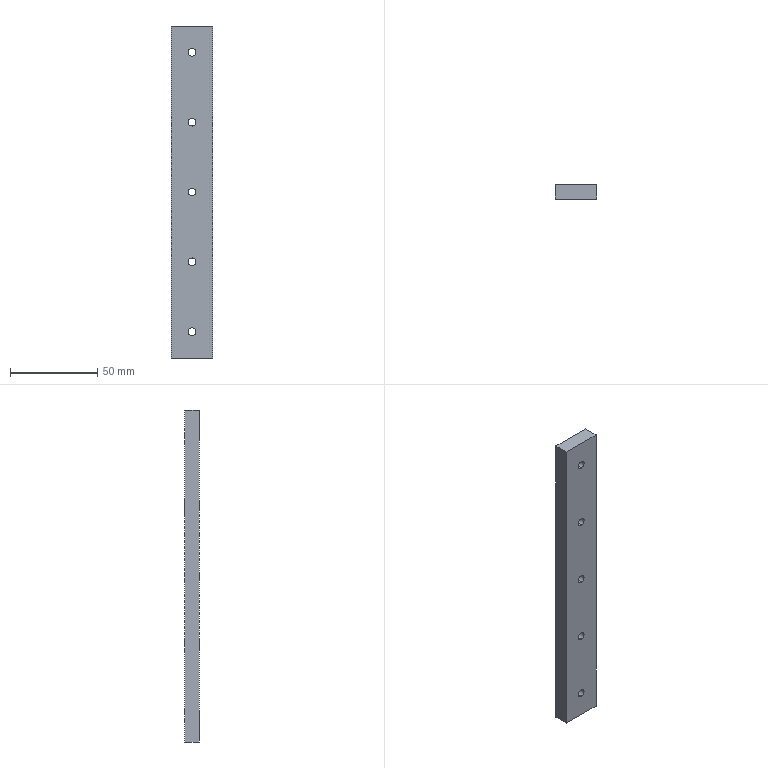Part | STEP file | 11-MGW12CR190Z0C11 | 1 solid | 31 faces | box 24 x 8.5 x 190 mm | volume 37397 mm3 | cylinder 20 | plane 11 | commonest cylinder face diameters 4.5 x10 8 x10
STEP:
#1=CARTESIAN_POINT('',(-44.741,27.003,12.75));
#2=VERTEX_POINT('',#1);
#3=CARTESIAN_POINT('',(-44.741,27.003,17.25));
#4=VERTEX_POINT('',#3);
#5=CARTESIAN_POINT('',(-44.741,27.003,15.));
#6=DIRECTION('',(0.,1.,0.));
#7=DIRECTION('',(0.,0.,1.));
#8=AXIS2_PLACEMENT_3D('',#5,#6,#7);
#9=CIRCLE('',#8,2.25);
#10=EDGE_CURVE('',#2,#4,#9,.T.);
#11=ORIENTED_EDGE('',*,*,#10,.F.);
#12=CARTESIAN_POINT('',(-44.741,31.503,12.75));
#13=VERTEX_POINT('',#12);
#14=CARTESIAN_POINT('',(-44.741,35.503,12.75));
#15=DIRECTION('',(0.,1.,0.));
#16=VECTOR('',#15,1000.);
#17=LINE('',#14,#16);
#18=EDGE_CURVE('',#2,#13,#17,.T.);
#19=ORIENTED_EDGE('',*,*,#18,.T.);
#20=CARTESIAN_POINT('',(-44.741,31.503,17.25));
#21=VERTEX_POINT('',#20);
#22=CARTESIAN_POINT('',(-44.741,31.503,15.));
#23=DIRECTION('',(0.,1.,0.));
#24=DIRECTION('',(0.,0.,1.));
#25=AXIS2_PLACEMENT_3D('',#22,#23,#24);
#26=CIRCLE('',#25,2.25);
#27=EDGE_CURVE('',#13,#21,#26,.T.);
#28=ORIENTED_EDGE('',*,*,#27,.T.);
#29=CARTESIAN_POINT('',(-44.741,35.503,17.25));
#30=DIRECTION('',(0.,1.,0.));
#31=VECTOR('',#30,1000.);
#32=LINE('',#29,#31);
#33=EDGE_CURVE('',#4,#21,#32,.T.);
#34=ORIENTED_EDGE('',*,*,#33,.F.);
#35=EDGE_LOOP('',(#11,#19,#28,#34));
#36=FACE_OUTER_BOUND('',#35,.T.);
#37=CARTESIAN_POINT('',(-44.741,35.503,15.));
#38=DIRECTION('',(0.,1.,0.));
#39=DIRECTION('',(0.,0.,1.));
#40=AXIS2_PLACEMENT_3D('',#37,#38,#39);
#41=CYLINDRICAL_SURFACE('',#40,2.25);
#42=ADVANCED_FACE('',(#36),#41,.F.);
#43=CARTESIAN_POINT('',(-44.741,31.503,11.));
#44=VERTEX_POINT('',#43);
#45=CARTESIAN_POINT('',(-44.741,31.503,19.));
#46=VERTEX_POINT('',#45);
#47=CARTESIAN_POINT('',(-44.741,31.503,15.));
#48=DIRECTION('',(0.,1.,0.));
#49=DIRECTION('',(0.,0.,1.));
#50=AXIS2_PLACEMENT_3D('',#47,#48,#49);
#51=CIRCLE('',#50,4.);
#52=EDGE_CURVE('',#44,#46,#51,.T.);
#53=ORIENTED_EDGE('',*,*,#52,.F.);
#54=CARTESIAN_POINT('',(-44.741,35.503,11.));
#55=VERTEX_POINT('',#54);
#56=CARTESIAN_POINT('',(-44.741,35.503,11.));
#57=DIRECTION('',(0.,1.,0.));
#58=VECTOR('',#57,1000.);
#59=LINE('',#56,#58);
#60=EDGE_CURVE('',#44,#55,#59,.T.);
#61=ORIENTED_EDGE('',*,*,#60,.T.);
#62=CARTESIAN_POINT('',(-44.741,35.503,19.));
#63=VERTEX_POINT('',#62);
#64=CARTESIAN_POINT('',(-44.741,35.503,15.));
#65=DIRECTION('',(0.,1.,0.));
#66=DIRECTION('',(0.,0.,1.));
#67=AXIS2_PLACEMENT_3D('',#64,#65,#66);
#68=CIRCLE('',#67,4.);
#69=EDGE_CURVE('',#55,#63,#68,.T.);
#70=ORIENTED_EDGE('',*,*,#69,.T.);
#71=CARTESIAN_POINT('',(-44.741,35.503,19.));
#72=DIRECTION('',(0.,1.,0.));
#73=VECTOR('',#72,1000.);
#74=LINE('',#71,#73);
#75=EDGE_CURVE('',#46,#63,#74,.T.);
#76=ORIENTED_EDGE('',*,*,#75,.F.);
#77=EDGE_LOOP('',(#53,#61,#70,#76));
#78=FACE_OUTER_BOUND('',#77,.T.);
#79=CARTESIAN_POINT('',(-44.741,35.503,15.));
#80=DIRECTION('',(0.,1.,0.));
#81=DIRECTION('',(0.,0.,1.));
#82=AXIS2_PLACEMENT_3D('',#79,#80,#81);
#83=CYLINDRICAL_SURFACE('',#82,4.);
#84=ADVANCED_FACE('',(#78),#83,.F.);
#85=CARTESIAN_POINT('',(-44.741,27.003,52.75));
#86=VERTEX_POINT('',#85);
#87=CARTESIAN_POINT('',(-44.741,27.003,57.25));
#88=VERTEX_POINT('',#87);
#89=CARTESIAN_POINT('',(-44.741,27.003,55.));
#90=DIRECTION('',(0.,1.,0.));
#91=DIRECTION('',(0.,0.,1.));
#92=AXIS2_PLACEMENT_3D('',#89,#90,#91);
#93=CIRCLE('',#92,2.25);
#94=EDGE_CURVE('',#86,#88,#93,.T.);
#95=ORIENTED_EDGE('',*,*,#94,.F.);
#96=CARTESIAN_POINT('',(-44.741,31.503,52.75));
#97=VERTEX_POINT('',#96);
#98=CARTESIAN_POINT('',(-44.741,35.503,52.75));
#99=DIRECTION('',(0.,1.,0.));
#100=VECTOR('',#99,1000.);
#101=LINE('',#98,#100);
#102=EDGE_CURVE('',#86,#97,#101,.T.);
#103=ORIENTED_EDGE('',*,*,#102,.T.);
#104=CARTESIAN_POINT('',(-44.741,31.503,57.25));
#105=VERTEX_POINT('',#104);
#106=CARTESIAN_POINT('',(-44.741,31.503,55.));
#107=DIRECTION('',(0.,1.,0.));
#108=DIRECTION('',(0.,0.,1.));
#109=AXIS2_PLACEMENT_3D('',#106,#107,#108);
#110=CIRCLE('',#109,2.25);
#111=EDGE_CURVE('',#97,#105,#110,.T.);
#112=ORIENTED_EDGE('',*,*,#111,.T.);
#113=CARTESIAN_POINT('',(-44.741,35.503,57.25));
#114=DIRECTION('',(0.,1.,0.));
#115=VECTOR('',#114,1000.);
#116=LINE('',#113,#115);
#117=EDGE_CURVE('',#88,#105,#116,.T.);
#118=ORIENTED_EDGE('',*,*,#117,.F.);
#119=EDGE_LOOP('',(#95,#103,#112,#118));
#120=FACE_OUTER_BOUND('',#119,.T.);
#121=CARTESIAN_POINT('',(-44.741,35.503,55.));
#122=DIRECTION('',(0.,1.,0.));
#123=DIRECTION('',(0.,0.,1.));
#124=AXIS2_PLACEMENT_3D('',#121,#122,#123);
#125=CYLINDRICAL_SURFACE('',#124,2.25);
#126=ADVANCED_FACE('',(#120),#125,.F.);
#127=CARTESIAN_POINT('',(-44.741,31.503,51.));
#128=VERTEX_POINT('',#127);
#129=CARTESIAN_POINT('',(-44.741,31.503,59.));
#130=VERTEX_POINT('',#129);
#131=CARTESIAN_POINT('',(-44.741,31.503,55.));
#132=DIRECTION('',(0.,1.,0.));
#133=DIRECTION('',(0.,0.,1.));
#134=AXIS2_PLACEMENT_3D('',#131,#132,#133);
#135=CIRCLE('',#134,4.);
#136=EDGE_CURVE('',#128,#130,#135,.T.);
#137=ORIENTED_EDGE('',*,*,#136,.F.);
#138=CARTESIAN_POINT('',(-44.741,35.503,51.));
#139=VERTEX_POINT('',#138);
#140=CARTESIAN_POINT('',(-44.741,35.503,51.));
#141=DIRECTION('',(0.,1.,0.));
#142=VECTOR('',#141,1000.);
#143=LINE('',#140,#142);
#144=EDGE_CURVE('',#128,#139,#143,.T.);
#145=ORIENTED_EDGE('',*,*,#144,.T.);
#146=CARTESIAN_POINT('',(-44.741,35.503,59.));
#147=VERTEX_POINT('',#146);
#148=CARTESIAN_POINT('',(-44.741,35.503,55.));
#149=DIRECTION('',(0.,1.,0.));
#150=DIRECTION('',(0.,0.,1.));
#151=AXIS2_PLACEMENT_3D('',#148,#149,#150);
#152=CIRCLE('',#151,4.);
#153=EDGE_CURVE('',#139,#147,#152,.T.);
#154=ORIENTED_EDGE('',*,*,#153,.T.);
#155=CARTESIAN_POINT('',(-44.741,35.503,59.));
#156=DIRECTION('',(0.,1.,0.));
#157=VECTOR('',#156,1000.);
#158=LINE('',#155,#157);
#159=EDGE_CURVE('',#130,#147,#158,.T.);
#160=ORIENTED_EDGE('',*,*,#159,.F.);
#161=EDGE_LOOP('',(#137,#145,#154,#160));
#162=FACE_OUTER_BOUND('',#161,.T.);
#163=CARTESIAN_POINT('',(-44.741,35.503,55.));
#164=DIRECTION('',(0.,1.,0.));
#165=DIRECTION('',(0.,0.,1.));
#166=AXIS2_PLACEMENT_3D('',#163,#164,#165);
#167=CYLINDRICAL_SURFACE('',#166,4.);
#168=ADVANCED_FACE('',(#162),#167,.F.);
#169=CARTESIAN_POINT('',(-44.741,27.003,92.75));
#170=VERTEX_POINT('',#169);
#171=CARTESIAN_POINT('',(-44.741,27.003,97.25));
#172=VERTEX_POINT('',#171);
#173=CARTESIAN_POINT('',(-44.741,27.003,95.));
#174=DIRECTION('',(0.,1.,0.));
#175=DIRECTION('',(0.,0.,1.));
#176=AXIS2_PLACEMENT_3D('',#173,#174,#175);
#177=CIRCLE('',#176,2.25);
#178=EDGE_CURVE('',#170,#172,#177,.T.);
#179=ORIENTED_EDGE('',*,*,#178,.F.);
#180=CARTESIAN_POINT('',(-44.741,31.503,92.75));
#181=VERTEX_POINT('',#180);
#182=CARTESIAN_POINT('',(-44.741,35.503,92.75));
#183=DIRECTION('',(0.,1.,0.));
#184=VECTOR('',#183,1000.);
#185=LINE('',#182,#184);
#186=EDGE_CURVE('',#170,#181,#185,.T.);
#187=ORIENTED_EDGE('',*,*,#186,.T.);
#188=CARTESIAN_POINT('',(-44.741,31.503,97.25));
#189=VERTEX_POINT('',#188);
#190=CARTESIAN_POINT('',(-44.741,31.503,95.));
#191=DIRECTION('',(0.,1.,0.));
#192=DIRECTION('',(0.,0.,1.));
#193=AXIS2_PLACEMENT_3D('',#190,#191,#192);
#194=CIRCLE('',#193,2.25);
#195=EDGE_CURVE('',#181,#189,#194,.T.);
#196=ORIENTED_EDGE('',*,*,#195,.T.);
#197=CARTESIAN_POINT('',(-44.741,35.503,97.25));
#198=DIRECTION('',(0.,1.,0.));
#199=VECTOR('',#198,1000.);
#200=LINE('',#197,#199);
#201=EDGE_CURVE('',#172,#189,#200,.T.);
#202=ORIENTED_EDGE('',*,*,#201,.F.);
#203=EDGE_LOOP('',(#179,#187,#196,#202));
#204=FACE_OUTER_BOUND('',#203,.T.);
#205=CARTESIAN_POINT('',(-44.741,35.503,95.));
#206=DIRECTION('',(0.,1.,0.));
#207=DIRECTION('',(0.,0.,1.));
#208=AXIS2_PLACEMENT_3D('',#205,#206,#207);
#209=CYLINDRICAL_SURFACE('',#208,2.25);
#210=ADVANCED_FACE('',(#204),#209,.F.);
#211=CARTESIAN_POINT('',(-44.741,31.503,91.));
#212=VERTEX_POINT('',#211);
#213=CARTESIAN_POINT('',(-44.741,31.503,99.));
#214=VERTEX_POINT('',#213);
#215=CARTESIAN_POINT('',(-44.741,31.503,95.));
#216=DIRECTION('',(0.,1.,0.));
#217=DIRECTION('',(0.,0.,1.));
#218=AXIS2_PLACEMENT_3D('',#215,#216,#217);
#219=CIRCLE('',#218,4.);
#220=EDGE_CURVE('',#212,#214,#219,.T.);
#221=ORIENTED_EDGE('',*,*,#220,.F.);
#222=CARTESIAN_POINT('',(-44.741,35.503,91.));
#223=VERTEX_POINT('',#222);
#224=CARTESIAN_POINT('',(-44.741,35.503,91.));
#225=DIRECTION('',(0.,1.,0.));
#226=VECTOR('',#225,1000.);
#227=LINE('',#224,#226);
#228=EDGE_CURVE('',#212,#223,#227,.T.);
#229=ORIENTED_EDGE('',*,*,#228,.T.);
#230=CARTESIAN_POINT('',(-44.741,35.503,99.));
#231=VERTEX_POINT('',#230);
#232=CARTESIAN_POINT('',(-44.741,35.503,95.));
#233=DIRECTION('',(0.,1.,0.));
#234=DIRECTION('',(0.,0.,1.));
#235=AXIS2_PLACEMENT_3D('',#232,#233,#234);
#236=CIRCLE('',#235,4.);
#237=EDGE_CURVE('',#223,#231,#236,.T.);
#238=ORIENTED_EDGE('',*,*,#237,.T.);
#239=CARTESIAN_POINT('',(-44.741,35.503,99.));
#240=DIRECTION('',(0.,1.,0.));
#241=VECTOR('',#240,1000.);
#242=LINE('',#239,#241);
#243=EDGE_CURVE('',#214,#231,#242,.T.);
#244=ORIENTED_EDGE('',*,*,#243,.F.);
#245=EDGE_LOOP('',(#221,#229,#238,#244));
#246=FACE_OUTER_BOUND('',#245,.T.);
#247=CARTESIAN_POINT('',(-44.741,35.503,95.));
#248=DIRECTION('',(0.,1.,0.));
#249=DIRECTION('',(0.,0.,1.));
#250=AXIS2_PLACEMENT_3D('',#247,#248,#249);
#251=CYLINDRICAL_SURFACE('',#250,4.);
#252=ADVANCED_FACE('',(#246),#251,.F.);
#253=CARTESIAN_POINT('',(-44.741,31.503,131.));
#254=VERTEX_POINT('',#253);
#255=CARTESIAN_POINT('',(-44.741,31.503,139.));
#256=VERTEX_POINT('',#255);
#257=CARTESIAN_POINT('',(-44.741,31.503,135.));
#258=DIRECTION('',(0.,1.,0.));
#259=DIRECTION('',(0.,0.,1.));
#260=AXIS2_PLACEMENT_3D('',#257,#258,#259);
#261=CIRCLE('',#260,4.);
#262=EDGE_CURVE('',#254,#256,#261,.T.);
#263=ORIENTED_EDGE('',*,*,#262,.F.);
#264=CARTESIAN_POINT('',(-44.741,35.503,131.));
#265=VERTEX_POINT('',#264);
#266=CARTESIAN_POINT('',(-44.741,35.503,131.));
#267=DIRECTION('',(0.,1.,0.));
#268=VECTOR('',#267,1000.);
#269=LINE('',#266,#268);
#270=EDGE_CURVE('',#254,#265,#269,.T.);
#271=ORIENTED_EDGE('',*,*,#270,.T.);
#272=CARTESIAN_POINT('',(-44.741,35.503,139.));
#273=VERTEX_POINT('',#272);
#274=CARTESIAN_POINT('',(-44.741,35.503,135.));
#275=DIRECTION('',(0.,1.,0.));
#276=DIRECTION('',(0.,0.,1.));
#277=AXIS2_PLACEMENT_3D('',#274,#275,#276);
#278=CIRCLE('',#277,4.);
#279=EDGE_CURVE('',#265,#273,#278,.T.);
#280=ORIENTED_EDGE('',*,*,#279,.T.);
#281=CARTESIAN_POINT('',(-44.741,35.503,139.));
#282=DIRECTION('',(0.,1.,0.));
#283=VECTOR('',#282,1000.);
#284=LINE('',#281,#283);
#285=EDGE_CURVE('',#256,#273,#284,.T.);
#286=ORIENTED_EDGE('',*,*,#285,.F.);
#287=EDGE_LOOP('',(#263,#271,#280,#286));
#288=FACE_OUTER_BOUND('',#287,.T.);
#289=CARTESIAN_POINT('',(-44.741,35.503,135.));
#290=DIRECTION('',(0.,1.,0.));
#291=DIRECTION('',(0.,0.,1.));
#292=AXIS2_PLACEMENT_3D('',#289,#290,#291);
#293=CYLINDRICAL_SURFACE('',#292,4.);
#294=ADVANCED_FACE('',(#288),#293,.F.);
#295=CARTESIAN_POINT('',(-44.741,27.003,132.75));
#296=VERTEX_POINT('',#295);
#297=CARTESIAN_POINT('',(-44.741,27.003,137.25));
#298=VERTEX_POINT('',#297);
#299=CARTESIAN_POINT('',(-44.741,27.003,135.));
#300=DIRECTION('',(0.,1.,0.));
#301=DIRECTION('',(0.,0.,1.));
#302=AXIS2_PLACEMENT_3D('',#299,#300,#301);
#303=CIRCLE('',#302,2.25);
#304=EDGE_CURVE('',#296,#298,#303,.T.);
#305=ORIENTED_EDGE('',*,*,#304,.F.);
#306=CARTESIAN_POINT('',(-44.741,31.503,132.75));
#307=VERTEX_POINT('',#306);
#308=CARTESIAN_POINT('',(-44.741,35.503,132.75));
#309=DIRECTION('',(0.,1.,0.));
#310=VECTOR('',#309,1000.);
#311=LINE('',#308,#310);
#312=EDGE_CURVE('',#296,#307,#311,.T.);
#313=ORIENTED_EDGE('',*,*,#312,.T.);
#314=CARTESIAN_POINT('',(-44.741,31.503,137.25));
#315=VERTEX_POINT('',#314);
#316=CARTESIAN_POINT('',(-44.741,31.503,135.));
#317=DIRECTION('',(0.,1.,0.));
#318=DIRECTION('',(0.,0.,1.));
#319=AXIS2_PLACEMENT_3D('',#316,#317,#318);
#320=CIRCLE('',#319,2.25);
#321=EDGE_CURVE('',#307,#315,#320,.T.);
#322=ORIENTED_EDGE('',*,*,#321,.T.);
#323=CARTESIAN_POINT('',(-44.741,35.503,137.25));
#324=DIRECTION('',(0.,1.,0.));
#325=VECTOR('',#324,1000.);
#326=LINE('',#323,#325);
#327=EDGE_CURVE('',#298,#315,#326,.T.);
#328=ORIENTED_EDGE('',*,*,#327,.F.);
#329=EDGE_LOOP('',(#305,#313,#322,#328));
#330=FACE_OUTER_BOUND('',#329,.T.);
#331=CARTESIAN_POINT('',(-44.741,35.503,135.));
#332=DIRECTION('',(0.,1.,0.));
#333=DIRECTION('',(0.,0.,1.));
#334=AXIS2_PLACEMENT_3D('',#331,#332,#333);
#335=CYLINDRICAL_SURFACE('',#334,2.25);
#336=ADVANCED_FACE('',(#330),#335,.F.);
#337=CARTESIAN_POINT('',(-44.741,31.503,171.));
#338=VERTEX_POINT('',#337);
#339=CARTESIAN_POINT('',(-44.741,31.503,179.));
#340=VERTEX_POINT('',#339);
#341=CARTESIAN_POINT('',(-44.741,31.503,175.));
#342=DIRECTION('',(0.,1.,0.));
#343=DIRECTION('',(0.,0.,1.));
#344=AXIS2_PLACEMENT_3D('',#341,#342,#343);
#345=CIRCLE('',#344,4.);
#346=EDGE_CURVE('',#338,#340,#345,.T.);
#347=ORIENTED_EDGE('',*,*,#346,.F.);
#348=CARTESIAN_POINT('',(-44.741,35.503,171.));
#349=VERTEX_POINT('',#348);
#350=CARTESIAN_POINT('',(-44.741,35.503,171.));
#351=DIRECTION('',(0.,1.,0.));
#352=VECTOR('',#351,1000.);
#353=LINE('',#350,#352);
#354=EDGE_CURVE('',#338,#349,#353,.T.);
#355=ORIENTED_EDGE('',*,*,#354,.T.);
#356=CARTESIAN_POINT('',(-44.741,35.503,179.));
#357=VERTEX_POINT('',#356);
#358=CARTESIAN_POINT('',(-44.741,35.503,175.));
#359=DIRECTION('',(0.,1.,0.));
#360=DIRECTION('',(0.,0.,1.));
#361=AXIS2_PLACEMENT_3D('',#358,#359,#360);
#362=CIRCLE('',#361,4.);
#363=EDGE_CURVE('',#349,#357,#362,.T.);
#364=ORIENTED_EDGE('',*,*,#363,.T.);
#365=CARTESIAN_POINT('',(-44.741,35.503,179.));
#366=DIRECTION('',(0.,1.,0.));
#367=VECTOR('',#366,1000.);
#368=LINE('',#365,#367);
#369=EDGE_CURVE('',#340,#357,#368,.T.);
#370=ORIENTED_EDGE('',*,*,#369,.F.);
#371=EDGE_LOOP('',(#347,#355,#364,#370));
#372=FACE_OUTER_BOUND('',#371,.T.);
#373=CARTESIAN_POINT('',(-44.741,35.503,175.));
#374=DIRECTION('',(0.,1.,0.));
#375=DIRECTION('',(0.,0.,1.));
#376=AXIS2_PLACEMENT_3D('',#373,#374,#375);
#377=CYLINDRICAL_SURFACE('',#376,4.);
#378=ADVANCED_FACE('',(#372),#377,.F.);
#379=CARTESIAN_POINT('',(-44.741,27.003,172.75));
#380=VERTEX_POINT('',#379);
#381=CARTESIAN_POINT('',(-44.741,27.003,177.25));
#382=VERTEX_POINT('',#381);
#383=CARTESIAN_POINT('',(-44.741,27.003,175.));
#384=DIRECTION('',(0.,1.,0.));
#385=DIRECTION('',(0.,0.,1.));
#386=AXIS2_PLACEMENT_3D('',#383,#384,#385);
#387=CIRCLE('',#386,2.25);
#388=EDGE_CURVE('',#380,#382,#387,.T.);
#389=ORIENTED_EDGE('',*,*,#388,.F.);
#390=CARTESIAN_POINT('',(-44.741,31.503,172.75));
#391=VERTEX_POINT('',#390);
#392=CARTESIAN_POINT('',(-44.741,35.503,172.75));
#393=DIRECTION('',(0.,1.,0.));
#394=VECTOR('',#393,1000.);
#395=LINE('',#392,#394);
#396=EDGE_CURVE('',#380,#391,#395,.T.);
#397=ORIENTED_EDGE('',*,*,#396,.T.);
#398=CARTESIAN_POINT('',(-44.741,31.503,177.25));
#399=VERTEX_POINT('',#398);
#400=CARTESIAN_POINT('',(-44.741,31.503,175.));
#401=DIRECTION('',(0.,1.,0.));
#402=DIRECTION('',(0.,0.,1.));
#403=AXIS2_PLACEMENT_3D('',#400,#401,#402);
#404=CIRCLE('',#403,2.25);
#405=EDGE_CURVE('',#391,#399,#404,.T.);
#406=ORIENTED_EDGE('',*,*,#405,.T.);
#407=CARTESIAN_POINT('',(-44.741,35.503,177.25));
#408=DIRECTION('',(0.,1.,0.));
#409=VECTOR('',#408,1000.);
#410=LINE('',#407,#409);
#411=EDGE_CURVE('',#382,#399,#410,.T.);
#412=ORIENTED_EDGE('',*,*,#411,.F.);
#413=EDGE_LOOP('',(#389,#397,#406,#412));
#414=FACE_OUTER_BOUND('',#413,.T.);
#415=CARTESIAN_POINT('',(-44.741,35.503,175.));
#416=DIRECTION('',(0.,1.,0.));
#417=DIRECTION('',(0.,0.,1.));
#418=AXIS2_PLACEMENT_3D('',#415,#416,#417);
#419=CYLINDRICAL_SURFACE('',#418,2.25);
#420=ADVANCED_FACE('',(#414),#419,.F.);
#421=CARTESIAN_POINT('',(-56.741,35.503,0.));
#422=VERTEX_POINT('',#421);
#423=CARTESIAN_POINT('',(-56.741,27.003,0.));
#424=VERTEX_POINT('',#423);
#425=CARTESIAN_POINT('',(-56.741,35.503,0.));
#426=DIRECTION('',(0.,-1.,0.));
#427=VECTOR('',#426,1000.);
#428=LINE('',#425,#427);
#429=EDGE_CURVE('',#422,#424,#428,.T.);
#430=ORIENTED_EDGE('',*,*,#429,.T.);
#431=CARTESIAN_POINT('',(-56.741,27.003,190.));
#432=VERTEX_POINT('',#431);
#433=CARTESIAN_POINT('',(-56.741,27.003,190.));
#434=DIRECTION('',(0.,0.,-1.));
#435=VECTOR('',#434,1000.);
#436=LINE('',#433,#435);
#437=EDGE_CURVE('',#432,#424,#436,.T.);
#438=ORIENTED_EDGE('',*,*,#437,.F.);
#439=CARTESIAN_POINT('',(-56.741,35.503,190.));
#440=VERTEX_POINT('',#439);
#441=CARTESIAN_POINT('',(-56.741,35.503,190.));
#442=DIRECTION('',(0.,-1.,0.));
#443=VECTOR('',#442,1000.);
#444=LINE('',#441,#443);
#445=EDGE_CURVE('',#440,#432,#444,.T.);
#446=ORIENTED_EDGE('',*,*,#445,.F.);
#447=CARTESIAN_POINT('',(-56.741,35.503,190.));
#448=DIRECTION('',(0.,0.,-1.));
#449=VECTOR('',#448,1000.);
#450=LINE('',#447,#449);
#451=EDGE_CURVE('',#440,#422,#450,.T.);
#452=ORIENTED_EDGE('',*,*,#451,.T.);
#453=EDGE_LOOP('',(#430,#438,#446,#452));
#454=FACE_OUTER_BOUND('',#453,.T.);
#455=CARTESIAN_POINT('',(-56.741,35.503,190.));
#456=DIRECTION('',(1.,0.,0.));
#457=DIRECTION('',(0.,1.,0.));
#458=AXIS2_PLACEMENT_3D('',#455,#456,#457);
#459=PLANE('',#458);
#460=ADVANCED_FACE('',(#454),#459,.F.);
#461=CARTESIAN_POINT('',(-44.741,27.003,135.));
#462=DIRECTION('',(0.,1.,0.));
#463=DIRECTION('',(0.,0.,1.));
#464=AXIS2_PLACEMENT_3D('',#461,#462,#463);
#465=CIRCLE('',#464,2.25);
#466=EDGE_CURVE('',#298,#296,#465,.T.);
#467=ORIENTED_EDGE('',*,*,#466,.T.);
#468=ORIENTED_EDGE('',*,*,#304,.T.);
#469=EDGE_LOOP('',(#467,#468));
#470=FACE_BOUND('',#469,.T.);
#471=CARTESIAN_POINT('',(-44.741,27.003,175.));
#472=DIRECTION('',(0.,1.,0.));
#473=DIRECTION('',(0.,0.,1.));
#474=AXIS2_PLACEMENT_3D('',#471,#472,#473);
#475=CIRCLE('',#474,2.25);
#476=EDGE_CURVE('',#382,#380,#475,.T.);
#477=ORIENTED_EDGE('',*,*,#476,.T.);
#478=ORIENTED_EDGE('',*,*,#388,.T.);
#479=EDGE_LOOP('',(#477,#478));
#480=FACE_BOUND('',#479,.T.);
#481=CARTESIAN_POINT('',(-32.741,27.003,0.));
#482=VERTEX_POINT('',#481);
#483=CARTESIAN_POINT('',(-56.741,27.003,0.));
#484=DIRECTION('',(1.,0.,0.));
#485=VECTOR('',#484,1000.);
#486=LINE('',#483,#485);
#487=EDGE_CURVE('',#424,#482,#486,.T.);
#488=ORIENTED_EDGE('',*,*,#487,.T.);
#489=CARTESIAN_POINT('',(-32.741,27.003,190.));
#490=VERTEX_POINT('',#489);
#491=CARTESIAN_POINT('',(-32.741,27.003,190.));
#492=DIRECTION('',(0.,0.,-1.));
#493=VECTOR('',#492,1000.);
#494=LINE('',#491,#493);
#495=EDGE_CURVE('',#490,#482,#494,.T.);
#496=ORIENTED_EDGE('',*,*,#495,.F.);
#497=CARTESIAN_POINT('',(-56.741,27.003,190.));
#498=DIRECTION('',(1.,0.,0.));
#499=VECTOR('',#498,1000.);
#500=LINE('',#497,#499);
#501=EDGE_CURVE('',#432,#490,#500,.T.);
#502=ORIENTED_EDGE('',*,*,#501,.F.);
#503=ORIENTED_EDGE('',*,*,#437,.T.);
#504=EDGE_LOOP('',(#488,#496,#502,#503));
#505=FACE_OUTER_BOUND('',#504,.T.);
#506=CARTESIAN_POINT('',(-44.741,27.003,95.));
#507=DIRECTION('',(0.,1.,0.));
#508=DIRECTION('',(0.,0.,1.));
#509=AXIS2_PLACEMENT_3D('',#506,#507,#508);
#510=CIRCLE('',#509,2.25);
#511=EDGE_CURVE('',#172,#170,#510,.T.);
#512=ORIENTED_EDGE('',*,*,#511,.T.);
#513=ORIENTED_EDGE('',*,*,#178,.T.);
#514=EDGE_LOOP('',(#512,#513));
#515=FACE_BOUND('',#514,.T.);
#516=CARTESIAN_POINT('',(-44.741,27.003,55.));
#517=DIRECTION('',(0.,1.,0.));
#518=DIRECTION('',(0.,0.,1.));
#519=AXIS2_PLACEMENT_3D('',#516,#517,#518);
#520=CIRCLE('',#519,2.25);
#521=EDGE_CURVE('',#88,#86,#520,.T.);
#522=ORIENTED_EDGE('',*,*,#521,.T.);
#523=ORIENTED_EDGE('',*,*,#94,.T.);
#524=EDGE_LOOP('',(#522,#523));
#525=FACE_BOUND('',#524,.T.);
#526=CARTESIAN_POINT('',(-44.741,27.003,15.));
#527=DIRECTION('',(0.,1.,0.));
#528=DIRECTION('',(0.,0.,1.));
#529=AXIS2_PLACEMENT_3D('',#526,#527,#528);
#530=CIRCLE('',#529,2.25);
#531=EDGE_CURVE('',#4,#2,#530,.T.);
#532=ORIENTED_EDGE('',*,*,#531,.T.);
#533=ORIENTED_EDGE('',*,*,#10,.T.);
#534=EDGE_LOOP('',(#532,#533));
#535=FACE_BOUND('',#534,.T.);
#536=CARTESIAN_POINT('',(-56.741,27.003,190.));
#537=DIRECTION('',(0.,1.,0.));
#538=DIRECTION('',(0.,0.,1.));
#539=AXIS2_PLACEMENT_3D('',#536,#537,#538);
#540=PLANE('',#539);
#541=ADVANCED_FACE('',(#470,#480,#505,#515,#525,#535),#540,.F.);
#542=CARTESIAN_POINT('',(-32.741,35.503,0.));
#543=VERTEX_POINT('',#542);
#544=CARTESIAN_POINT('',(-32.741,35.503,0.));
#545=DIRECTION('',(0.,1.,0.));
#546=VECTOR('',#545,1000.);
#547=LINE('',#544,#546);
#548=EDGE_CURVE('',#482,#543,#547,.T.);
#549=ORIENTED_EDGE('',*,*,#548,.T.);
#550=CARTESIAN_POINT('',(-32.741,35.503,190.));
#551=VERTEX_POINT('',#550);
#552=CARTESIAN_POINT('',(-32.741,35.503,190.));
#553=DIRECTION('',(0.,0.,-1.));
#554=VECTOR('',#553,1000.);
#555=LINE('',#552,#554);
#556=EDGE_CURVE('',#551,#543,#555,.T.);
#557=ORIENTED_EDGE('',*,*,#556,.F.);
#558=CARTESIAN_POINT('',(-32.741,35.503,190.));
#559=DIRECTION('',(0.,1.,0.));
#560=VECTOR('',#559,1000.);
#561=LINE('',#558,#560);
#562=EDGE_CURVE('',#490,#551,#561,.T.);
#563=ORIENTED_EDGE('',*,*,#562,.F.);
#564=ORIENTED_EDGE('',*,*,#495,.T.);
#565=EDGE_LOOP('',(#549,#557,#563,#564));
#566=FACE_OUTER_BOUND('',#565,.T.);
#567=CARTESIAN_POINT('',(-32.741,35.503,190.));
#568=DIRECTION('',(-1.,0.,0.));
#569=DIRECTION('',(0.,0.,1.));
#570=AXIS2_PLACEMENT_3D('',#567,#568,#569);
#571=PLANE('',#570);
#572=ADVANCED_FACE('',(#566),#571,.F.);
#573=CARTESIAN_POINT('',(-44.741,35.503,135.));
#574=DIRECTION('',(0.,1.,0.));
#575=DIRECTION('',(0.,0.,1.));
#576=AXIS2_PLACEMENT_3D('',#573,#574,#575);
#577=CIRCLE('',#576,4.);
#578=EDGE_CURVE('',#273,#265,#577,.T.);
#579=ORIENTED_EDGE('',*,*,#578,.F.);
#580=ORIENTED_EDGE('',*,*,#279,.F.);
#581=EDGE_LOOP('',(#579,#580));
#582=FACE_BOUND('',#581,.T.);
#583=CARTESIAN_POINT('',(-44.741,35.503,175.));
#584=DIRECTION('',(0.,1.,0.));
#585=DIRECTION('',(0.,0.,1.));
#586=AXIS2_PLACEMENT_3D('',#583,#584,#585);
#587=CIRCLE('',#586,4.);
#588=EDGE_CURVE('',#357,#349,#587,.T.);
#589=ORIENTED_EDGE('',*,*,#588,.F.);
#590=ORIENTED_EDGE('',*,*,#363,.F.);
#591=EDGE_LOOP('',(#589,#590));
#592=FACE_BOUND('',#591,.T.);
#593=CARTESIAN_POINT('',(-56.741,35.503,0.));
#594=DIRECTION('',(-1.,0.,0.));
#595=VECTOR('',#594,1000.);
#596=LINE('',#593,#595);
#597=EDGE_CURVE('',#543,#422,#596,.T.);
#598=ORIENTED_EDGE('',*,*,#597,.T.);
#599=ORIENTED_EDGE('',*,*,#451,.F.);
#600=CARTESIAN_POINT('',(-56.741,35.503,190.));
#601=DIRECTION('',(-1.,0.,0.));
#602=VECTOR('',#601,1000.);
#603=LINE('',#600,#602);
#604=EDGE_CURVE('',#551,#440,#603,.T.);
#605=ORIENTED_EDGE('',*,*,#604,.F.);
#606=ORIENTED_EDGE('',*,*,#556,.T.);
#607=EDGE_LOOP('',(#598,#599,#605,#606));
#608=FACE_OUTER_BOUND('',#607,.T.);
#609=CARTESIAN_POINT('',(-44.741,35.503,95.));
#610=DIRECTION('',(0.,1.,0.));
#611=DIRECTION('',(0.,0.,1.));
#612=AXIS2_PLACEMENT_3D('',#609,#610,#611);
#613=CIRCLE('',#612,4.);
#614=EDGE_CURVE('',#231,#223,#613,.T.);
#615=ORIENTED_EDGE('',*,*,#614,.F.);
#616=ORIENTED_EDGE('',*,*,#237,.F.);
#617=EDGE_LOOP('',(#615,#616));
#618=FACE_BOUND('',#617,.T.);
#619=CARTESIAN_POINT('',(-44.741,35.503,55.));
#620=DIRECTION('',(0.,1.,0.));
#621=DIRECTION('',(0.,0.,1.));
#622=AXIS2_PLACEMENT_3D('',#619,#620,#621);
#623=CIRCLE('',#622,4.);
#624=EDGE_CURVE('',#147,#139,#623,.T.);
#625=ORIENTED_EDGE('',*,*,#624,.F.);
#626=ORIENTED_EDGE('',*,*,#153,.F.);
#627=EDGE_LOOP('',(#625,#626));
#628=FACE_BOUND('',#627,.T.);
#629=CARTESIAN_POINT('',(-44.741,35.503,15.));
#630=DIRECTION('',(0.,1.,0.));
#631=DIRECTION('',(0.,0.,1.));
#632=AXIS2_PLACEMENT_3D('',#629,#630,#631);
#633=CIRCLE('',#632,4.);
#634=EDGE_CURVE('',#63,#55,#633,.T.);
#635=ORIENTED_EDGE('',*,*,#634,.F.);
#636=ORIENTED_EDGE('',*,*,#69,.F.);
#637=EDGE_LOOP('',(#635,#636));
#638=FACE_BOUND('',#637,.T.);
#639=CARTESIAN_POINT('',(-56.741,35.503,190.));
#640=DIRECTION('',(0.,-1.,0.));
#641=DIRECTION('',(0.,0.,-1.));
#642=AXIS2_PLACEMENT_3D('',#639,#640,#641);
#643=PLANE('',#642);
#644=ADVANCED_FACE('',(#582,#592,#608,#618,#628,#638),#643,.F.);
#645=ORIENTED_EDGE('',*,*,#445,.T.);
#646=ORIENTED_EDGE('',*,*,#501,.T.);
#647=ORIENTED_EDGE('',*,*,#562,.T.);
#648=ORIENTED_EDGE('',*,*,#604,.T.);
#649=EDGE_LOOP('',(#645,#646,#647,#648));
#650=FACE_OUTER_BOUND('',#649,.T.);
#651=CARTESIAN_POINT('',(-56.741,27.003,190.));
#652=DIRECTION('',(0.,0.,1.));
#653=DIRECTION('',(1.,0.,0.));
#654=AXIS2_PLACEMENT_3D('',#651,#652,#653);
#655=PLANE('',#654);
#656=ADVANCED_FACE('',(#650),#655,.T.);
#657=ORIENTED_EDGE('',*,*,#429,.F.);
#658=ORIENTED_EDGE('',*,*,#597,.F.);
#659=ORIENTED_EDGE('',*,*,#548,.F.);
#660=ORIENTED_EDGE('',*,*,#487,.F.);
#661=EDGE_LOOP('',(#657,#658,#659,#660));
#662=FACE_OUTER_BOUND('',#661,.T.);
#663=CARTESIAN_POINT('',(-56.741,27.003,0.));
#664=DIRECTION('',(0.,0.,1.));
#665=DIRECTION('',(1.,0.,0.));
#666=AXIS2_PLACEMENT_3D('',#663,#664,#665);
#667=PLANE('',#666);
#668=ADVANCED_FACE('',(#662),#667,.F.);
#669=ORIENTED_EDGE('',*,*,#396,.F.);
#670=ORIENTED_EDGE('',*,*,#476,.F.);
#671=ORIENTED_EDGE('',*,*,#411,.T.);
#672=CARTESIAN_POINT('',(-44.741,31.503,175.));
#673=DIRECTION('',(0.,1.,0.));
#674=DIRECTION('',(0.,0.,1.));
#675=AXIS2_PLACEMENT_3D('',#672,#673,#674);
#676=CIRCLE('',#675,2.25);
#677=EDGE_CURVE('',#399,#391,#676,.T.);
#678=ORIENTED_EDGE('',*,*,#677,.T.);
#679=EDGE_LOOP('',(#669,#670,#671,#678));
#680=FACE_OUTER_BOUND('',#679,.T.);
#681=CARTESIAN_POINT('',(-44.741,35.503,175.));
#682=DIRECTION('',(0.,1.,0.));
#683=DIRECTION('',(0.,0.,1.));
#684=AXIS2_PLACEMENT_3D('',#681,#682,#683);
#685=CYLINDRICAL_SURFACE('',#684,2.25);
#686=ADVANCED_FACE('',(#680),#685,.F.);
#687=ORIENTED_EDGE('',*,*,#677,.F.);
#688=ORIENTED_EDGE('',*,*,#405,.F.);
#689=EDGE_LOOP('',(#687,#688));
#690=FACE_BOUND('',#689,.T.);
#691=CARTESIAN_POINT('',(-44.741,31.503,175.));
#692=DIRECTION('',(0.,1.,0.));
#693=DIRECTION('',(0.,0.,1.));
#694=AXIS2_PLACEMENT_3D('',#691,#692,#693);
#695=CIRCLE('',#694,4.);
#696=EDGE_CURVE('',#340,#338,#695,.T.);
#697=ORIENTED_EDGE('',*,*,#696,.T.);
#698=ORIENTED_EDGE('',*,*,#346,.T.);
#699=EDGE_LOOP('',(#697,#698));
#700=FACE_OUTER_BOUND('',#699,.T.);
#701=CARTESIAN_POINT('',(-42.491,31.503,175.));
#702=DIRECTION('',(0.,-1.,0.));
#703=DIRECTION('',(0.,0.,-1.));
#704=AXIS2_PLACEMENT_3D('',#701,#702,#703);
#705=PLANE('',#704);
#706=ADVANCED_FACE('',(#690,#700),#705,.F.);
#707=ORIENTED_EDGE('',*,*,#354,.F.);
#708=ORIENTED_EDGE('',*,*,#696,.F.);
#709=ORIENTED_EDGE('',*,*,#369,.T.);
#710=ORIENTED_EDGE('',*,*,#588,.T.);
#711=EDGE_LOOP('',(#707,#708,#709,#710));
#712=FACE_OUTER_BOUND('',#711,.T.);
#713=CARTESIAN_POINT('',(-44.741,35.503,175.));
#714=DIRECTION('',(0.,1.,0.));
#715=DIRECTION('',(0.,0.,1.));
#716=AXIS2_PLACEMENT_3D('',#713,#714,#715);
#717=CYLINDRICAL_SURFACE('',#716,4.);
#718=ADVANCED_FACE('',(#712),#717,.F.);
#719=ORIENTED_EDGE('',*,*,#270,.F.);
#720=CARTESIAN_POINT('',(-44.741,31.503,135.));
#721=DIRECTION('',(0.,1.,0.));
#722=DIRECTION('',(0.,0.,1.));
#723=AXIS2_PLACEMENT_3D('',#720,#721,#722);
#724=CIRCLE('',#723,4.);
#725=EDGE_CURVE('',#256,#254,#724,.T.);
#726=ORIENTED_EDGE('',*,*,#725,.F.);
#727=ORIENTED_EDGE('',*,*,#285,.T.);
#728=ORIENTED_EDGE('',*,*,#578,.T.);
#729=EDGE_LOOP('',(#719,#726,#727,#728));
#730=FACE_OUTER_BOUND('',#729,.T.);
#731=CARTESIAN_POINT('',(-44.741,35.503,135.));
#732=DIRECTION('',(0.,1.,0.));
#733=DIRECTION('',(0.,0.,1.));
#734=AXIS2_PLACEMENT_3D('',#731,#732,#733);
#735=CYLINDRICAL_SURFACE('',#734,4.);
#736=ADVANCED_FACE('',(#730),#735,.F.);
#737=CARTESIAN_POINT('',(-44.741,31.503,135.));
#738=DIRECTION('',(0.,1.,0.));
#739=DIRECTION('',(0.,0.,1.));
#740=AXIS2_PLACEMENT_3D('',#737,#738,#739);
#741=CIRCLE('',#740,2.25);
#742=EDGE_CURVE('',#315,#307,#741,.T.);
#743=ORIENTED_EDGE('',*,*,#742,.F.);
#744=ORIENTED_EDGE('',*,*,#321,.F.);
#745=EDGE_LOOP('',(#743,#744));
#746=FACE_BOUND('',#745,.T.);
#747=ORIENTED_EDGE('',*,*,#725,.T.);
#748=ORIENTED_EDGE('',*,*,#262,.T.);
#749=EDGE_LOOP('',(#747,#748));
#750=FACE_OUTER_BOUND('',#749,.T.);
#751=CARTESIAN_POINT('',(-42.491,31.503,135.));
#752=DIRECTION('',(0.,-1.,0.));
#753=DIRECTION('',(0.,0.,-1.));
#754=AXIS2_PLACEMENT_3D('',#751,#752,#753);
#755=PLANE('',#754);
#756=ADVANCED_FACE('',(#746,#750),#755,.F.);
#757=ORIENTED_EDGE('',*,*,#312,.F.);
#758=ORIENTED_EDGE('',*,*,#466,.F.);
#759=ORIENTED_EDGE('',*,*,#327,.T.);
#760=ORIENTED_EDGE('',*,*,#742,.T.);
#761=EDGE_LOOP('',(#757,#758,#759,#760));
#762=FACE_OUTER_BOUND('',#761,.T.);
#763=CARTESIAN_POINT('',(-44.741,35.503,135.));
#764=DIRECTION('',(0.,1.,0.));
#765=DIRECTION('',(0.,0.,1.));
#766=AXIS2_PLACEMENT_3D('',#763,#764,#765);
#767=CYLINDRICAL_SURFACE('',#766,2.25);
#768=ADVANCED_FACE('',(#762),#767,.F.);
#769=ORIENTED_EDGE('',*,*,#228,.F.);
#770=CARTESIAN_POINT('',(-44.741,31.503,95.));
#771=DIRECTION('',(0.,1.,0.));
#772=DIRECTION('',(0.,0.,1.));
#773=AXIS2_PLACEMENT_3D('',#770,#771,#772);
#774=CIRCLE('',#773,4.);
#775=EDGE_CURVE('',#214,#212,#774,.T.);
#776=ORIENTED_EDGE('',*,*,#775,.F.);
#777=ORIENTED_EDGE('',*,*,#243,.T.);
#778=ORIENTED_EDGE('',*,*,#614,.T.);
#779=EDGE_LOOP('',(#769,#776,#777,#778));
#780=FACE_OUTER_BOUND('',#779,.T.);
#781=CARTESIAN_POINT('',(-44.741,35.503,95.));
#782=DIRECTION('',(0.,1.,0.));
#783=DIRECTION('',(0.,0.,1.));
#784=AXIS2_PLACEMENT_3D('',#781,#782,#783);
#785=CYLINDRICAL_SURFACE('',#784,4.);
#786=ADVANCED_FACE('',(#780),#785,.F.);
#787=CARTESIAN_POINT('',(-44.741,31.503,95.));
#788=DIRECTION('',(0.,1.,0.));
#789=DIRECTION('',(0.,0.,1.));
#790=AXIS2_PLACEMENT_3D('',#787,#788,#789);
#791=CIRCLE('',#790,2.25);
#792=EDGE_CURVE('',#189,#181,#791,.T.);
#793=ORIENTED_EDGE('',*,*,#792,.F.);
#794=ORIENTED_EDGE('',*,*,#195,.F.);
#795=EDGE_LOOP('',(#793,#794));
#796=FACE_BOUND('',#795,.T.);
#797=ORIENTED_EDGE('',*,*,#775,.T.);
#798=ORIENTED_EDGE('',*,*,#220,.T.);
#799=EDGE_LOOP('',(#797,#798));
#800=FACE_OUTER_BOUND('',#799,.T.);
#801=CARTESIAN_POINT('',(-42.491,31.503,95.));
#802=DIRECTION('',(0.,-1.,0.));
#803=DIRECTION('',(0.,0.,-1.));
#804=AXIS2_PLACEMENT_3D('',#801,#802,#803);
#805=PLANE('',#804);
#806=ADVANCED_FACE('',(#796,#800),#805,.F.);
#807=ORIENTED_EDGE('',*,*,#186,.F.);
#808=ORIENTED_EDGE('',*,*,#511,.F.);
#809=ORIENTED_EDGE('',*,*,#201,.T.);
#810=ORIENTED_EDGE('',*,*,#792,.T.);
#811=EDGE_LOOP('',(#807,#808,#809,#810));
#812=FACE_OUTER_BOUND('',#811,.T.);
#813=CARTESIAN_POINT('',(-44.741,35.503,95.));
#814=DIRECTION('',(0.,1.,0.));
#815=DIRECTION('',(0.,0.,1.));
#816=AXIS2_PLACEMENT_3D('',#813,#814,#815);
#817=CYLINDRICAL_SURFACE('',#816,2.25);
#818=ADVANCED_FACE('',(#812),#817,.F.);
#819=ORIENTED_EDGE('',*,*,#144,.F.);
#820=CARTESIAN_POINT('',(-44.741,31.503,55.));
#821=DIRECTION('',(0.,1.,0.));
#822=DIRECTION('',(0.,0.,1.));
#823=AXIS2_PLACEMENT_3D('',#820,#821,#822);
#824=CIRCLE('',#823,4.);
#825=EDGE_CURVE('',#130,#128,#824,.T.);
#826=ORIENTED_EDGE('',*,*,#825,.F.);
#827=ORIENTED_EDGE('',*,*,#159,.T.);
#828=ORIENTED_EDGE('',*,*,#624,.T.);
#829=EDGE_LOOP('',(#819,#826,#827,#828));
#830=FACE_OUTER_BOUND('',#829,.T.);
#831=CARTESIAN_POINT('',(-44.741,35.503,55.));
#832=DIRECTION('',(0.,1.,0.));
#833=DIRECTION('',(0.,0.,1.));
#834=AXIS2_PLACEMENT_3D('',#831,#832,#833);
#835=CYLINDRICAL_SURFACE('',#834,4.);
#836=ADVANCED_FACE('',(#830),#835,.F.);
#837=CARTESIAN_POINT('',(-44.741,31.503,55.));
#838=DIRECTION('',(0.,1.,0.));
#839=DIRECTION('',(0.,0.,1.));
#840=AXIS2_PLACEMENT_3D('',#837,#838,#839);
#841=CIRCLE('',#840,2.25);
#842=EDGE_CURVE('',#105,#97,#841,.T.);
#843=ORIENTED_EDGE('',*,*,#842,.F.);
#844=ORIENTED_EDGE('',*,*,#111,.F.);
#845=EDGE_LOOP('',(#843,#844));
#846=FACE_BOUND('',#845,.T.);
#847=ORIENTED_EDGE('',*,*,#825,.T.);
#848=ORIENTED_EDGE('',*,*,#136,.T.);
#849=EDGE_LOOP('',(#847,#848));
#850=FACE_OUTER_BOUND('',#849,.T.);
#851=CARTESIAN_POINT('',(-42.491,31.503,55.));
#852=DIRECTION('',(0.,-1.,0.));
#853=DIRECTION('',(0.,0.,-1.));
#854=AXIS2_PLACEMENT_3D('',#851,#852,#853);
#855=PLANE('',#854);
#856=ADVANCED_FACE('',(#846,#850),#855,.F.);
#857=ORIENTED_EDGE('',*,*,#102,.F.);
#858=ORIENTED_EDGE('',*,*,#521,.F.);
#859=ORIENTED_EDGE('',*,*,#117,.T.);
#860=ORIENTED_EDGE('',*,*,#842,.T.);
#861=EDGE_LOOP('',(#857,#858,#859,#860));
#862=FACE_OUTER_BOUND('',#861,.T.);
#863=CARTESIAN_POINT('',(-44.741,35.503,55.));
#864=DIRECTION('',(0.,1.,0.));
#865=DIRECTION('',(0.,0.,1.));
#866=AXIS2_PLACEMENT_3D('',#863,#864,#865);
#867=CYLINDRICAL_SURFACE('',#866,2.25);
#868=ADVANCED_FACE('',(#862),#867,.F.);
#869=ORIENTED_EDGE('',*,*,#60,.F.);
#870=CARTESIAN_POINT('',(-44.741,31.503,15.));
#871=DIRECTION('',(0.,1.,0.));
#872=DIRECTION('',(0.,0.,1.));
#873=AXIS2_PLACEMENT_3D('',#870,#871,#872);
#874=CIRCLE('',#873,4.);
#875=EDGE_CURVE('',#46,#44,#874,.T.);
#876=ORIENTED_EDGE('',*,*,#875,.F.);
#877=ORIENTED_EDGE('',*,*,#75,.T.);
#878=ORIENTED_EDGE('',*,*,#634,.T.);
#879=EDGE_LOOP('',(#869,#876,#877,#878));
#880=FACE_OUTER_BOUND('',#879,.T.);
#881=CARTESIAN_POINT('',(-44.741,35.503,15.));
#882=DIRECTION('',(0.,1.,0.));
#883=DIRECTION('',(0.,0.,1.));
#884=AXIS2_PLACEMENT_3D('',#881,#882,#883);
#885=CYLINDRICAL_SURFACE('',#884,4.);
#886=ADVANCED_FACE('',(#880),#885,.F.);
#887=CARTESIAN_POINT('',(-44.741,31.503,15.));
#888=DIRECTION('',(0.,1.,0.));
#889=DIRECTION('',(0.,0.,1.));
#890=AXIS2_PLACEMENT_3D('',#887,#888,#889);
#891=CIRCLE('',#890,2.25);
#892=EDGE_CURVE('',#21,#13,#891,.T.);
#893=ORIENTED_EDGE('',*,*,#892,.F.);
#894=ORIENTED_EDGE('',*,*,#27,.F.);
#895=EDGE_LOOP('',(#893,#894));
#896=FACE_BOUND('',#895,.T.);
#897=ORIENTED_EDGE('',*,*,#875,.T.);
#898=ORIENTED_EDGE('',*,*,#52,.T.);
#899=EDGE_LOOP('',(#897,#898));
#900=FACE_OUTER_BOUND('',#899,.T.);
#901=CARTESIAN_POINT('',(-42.491,31.503,15.));
#902=DIRECTION('',(0.,-1.,0.));
#903=DIRECTION('',(0.,0.,-1.));
#904=AXIS2_PLACEMENT_3D('',#901,#902,#903);
#905=PLANE('',#904);
#906=ADVANCED_FACE('',(#896,#900),#905,.F.);
#907=ORIENTED_EDGE('',*,*,#18,.F.);
#908=ORIENTED_EDGE('',*,*,#531,.F.);
#909=ORIENTED_EDGE('',*,*,#33,.T.);
#910=ORIENTED_EDGE('',*,*,#892,.T.);
#911=EDGE_LOOP('',(#907,#908,#909,#910));
#912=FACE_OUTER_BOUND('',#911,.T.);
#913=CARTESIAN_POINT('',(-44.741,35.503,15.));
#914=DIRECTION('',(0.,1.,0.));
#915=DIRECTION('',(0.,0.,1.));
#916=AXIS2_PLACEMENT_3D('',#913,#914,#915);
#917=CYLINDRICAL_SURFACE('',#916,2.25);
#918=ADVANCED_FACE('',(#912),#917,.F.);
#919=CLOSED_SHELL('',(#42,#84,#126,#168,#210,#252,#294,#336,#378,#420,#460,#541,#572,#644,#656,#668,#686,#706,#718,#736,#756,#768,#786,#806,#818,#836,#856,#868,#886,#906,#918));
#920=MANIFOLD_SOLID_BREP('',#919);
#921=CARTESIAN_POINT('',(0.,0.,0.));
#922=DIRECTION('',(0.,0.,1.));
#923=DIRECTION('',(1.,0.,0.));
#924=AXIS2_PLACEMENT_3D('',#921,#922,#923);
#925=(LENGTH_UNIT()NAMED_UNIT(*)SI_UNIT(.MILLI.,.METRE.));
#926=UNCERTAINTY_MEASURE_WITH_UNIT(LENGTH_MEASURE(0.00001),#925,'','');
#927=(NAMED_UNIT(*)PLANE_ANGLE_UNIT()SI_UNIT($,.RADIAN.));
#928=(NAMED_UNIT(*)SI_UNIT($,.STERADIAN.)SOLID_ANGLE_UNIT());
#929=(GEOMETRIC_REPRESENTATION_CONTEXT(3)GLOBAL_UNCERTAINTY_ASSIGNED_CONTEXT((#926))GLOBAL_UNIT_ASSIGNED_CONTEXT((#925,#927,#928))REPRESENTATION_CONTEXT('',''));
#930=ADVANCED_BREP_SHAPE_REPRESENTATION('',(#920,#924),#929);